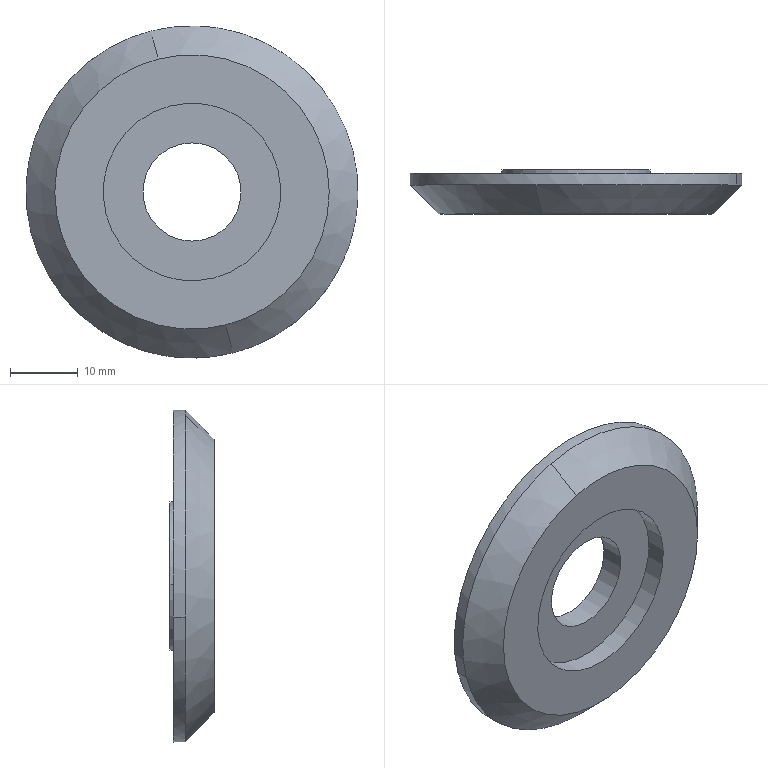Part | SolidWorks | features BaseBody 1 | 1 solid | 14 faces | box 49 x 6.5 x 49 mm | volume 7995 mm3 | cylinder 8 | plane 4 | cone 2 | commonest cylinder face diameters 14.5 x2 22 x2 26.2 x2 49 x2
STEP:
#1=CARTESIAN_POINT('',(-525.322,-118.5,-1.324));
#2=VERTEX_POINT('',#1);
#3=CARTESIAN_POINT('',(-535.321,-118.5,37.907));
#4=VERTEX_POINT('',#3);
#5=CARTESIAN_POINT('',(-530.322,-118.5,18.291));
#6=DIRECTION('',(0.,-1.,0.));
#7=DIRECTION('',(0.,0.,-1.));
#8=AXIS2_PLACEMENT_3D('',#5,#6,#7);
#9=CIRCLE('',#8,20.243);
#10=EDGE_CURVE('',#2,#4,#9,.T.);
#11=ORIENTED_EDGE('',*,*,#10,.F.);
#12=CARTESIAN_POINT('',(-524.27,-114.243,-5.45));
#13=VERTEX_POINT('',#12);
#14=CARTESIAN_POINT('',(-525.475,-119.121,-0.7223));
#15=DIRECTION('',(0.1747,0.7071,-0.6852));
#16=VECTOR('',#15,1000.);
#17=LINE('',#14,#16);
#18=EDGE_CURVE('',#2,#13,#17,.T.);
#19=ORIENTED_EDGE('',*,*,#18,.T.);
#20=CARTESIAN_POINT('',(-506.581,-114.243,24.343));
#21=VERTEX_POINT('',#20);
#22=CARTESIAN_POINT('',(-530.322,-114.243,18.291));
#23=DIRECTION('',(0.,1.,0.));
#24=DIRECTION('',(0.,0.,1.));
#25=AXIS2_PLACEMENT_3D('',#22,#23,#24);
#26=CIRCLE('',#25,24.5);
#27=EDGE_CURVE('',#21,#13,#26,.T.);
#28=ORIENTED_EDGE('',*,*,#27,.F.);
#29=CARTESIAN_POINT('',(-536.373,-114.243,42.032));
#30=VERTEX_POINT('',#29);
#31=CARTESIAN_POINT('',(-530.322,-114.243,18.291));
#32=DIRECTION('',(0.,1.,0.));
#33=DIRECTION('',(0.,0.,1.));
#34=AXIS2_PLACEMENT_3D('',#31,#32,#33);
#35=CIRCLE('',#34,24.5);
#36=EDGE_CURVE('',#30,#21,#35,.T.);
#37=ORIENTED_EDGE('',*,*,#36,.F.);
#38=CARTESIAN_POINT('',(-535.168,-119.121,37.304));
#39=DIRECTION('',(-0.1747,0.7071,0.6852));
#40=VECTOR('',#39,1000.);
#41=LINE('',#38,#40);
#42=EDGE_CURVE('',#4,#30,#41,.T.);
#43=ORIENTED_EDGE('',*,*,#42,.F.);
#44=EDGE_LOOP('',(#11,#19,#28,#37,#43));
#45=FACE_OUTER_BOUND('',#44,.T.);
#46=CARTESIAN_POINT('',(-530.322,-119.121,18.291));
#47=DIRECTION('',(0.,1.,0.));
#48=DIRECTION('',(-0.247,0.,0.969));
#49=AXIS2_PLACEMENT_3D('',#46,#47,#48);
#50=CONICAL_SURFACE('',#49,19.621,0.7854);
#51=ADVANCED_FACE('',(#45),#50,.T.);
#52=CARTESIAN_POINT('',(-537.528,-112.,17.495));
#53=VERTEX_POINT('',#52);
#54=CARTESIAN_POINT('',(-523.115,-112.,19.087));
#55=VERTEX_POINT('',#54);
#56=CARTESIAN_POINT('',(-530.322,-112.,18.291));
#57=DIRECTION('',(0.,1.,0.));
#58=DIRECTION('',(-0.994,0.,-0.1097));
#59=AXIS2_PLACEMENT_3D('',#56,#57,#58);
#60=CIRCLE('',#59,7.25);
#61=EDGE_CURVE('',#53,#55,#60,.T.);
#62=ORIENTED_EDGE('',*,*,#61,.T.);
#63=CARTESIAN_POINT('',(-523.115,-115.5,19.087));
#64=VERTEX_POINT('',#63);
#65=CARTESIAN_POINT('',(-523.115,-112.,19.087));
#66=DIRECTION('',(0.,-1.,0.));
#67=VECTOR('',#66,1000.);
#68=LINE('',#65,#67);
#69=EDGE_CURVE('',#55,#64,#68,.T.);
#70=ORIENTED_EDGE('',*,*,#69,.T.);
#71=CARTESIAN_POINT('',(-537.528,-115.5,17.495));
#72=VERTEX_POINT('',#71);
#73=CARTESIAN_POINT('',(-530.322,-115.5,18.291));
#74=DIRECTION('',(0.,-1.,0.));
#75=DIRECTION('',(0.969,0.,0.247));
#76=AXIS2_PLACEMENT_3D('',#73,#74,#75);
#77=CIRCLE('',#76,7.25);
#78=EDGE_CURVE('',#64,#72,#77,.T.);
#79=ORIENTED_EDGE('',*,*,#78,.T.);
#80=CARTESIAN_POINT('',(-537.528,-112.,17.495));
#81=DIRECTION('',(0.,-1.,0.));
#82=VECTOR('',#81,1000.);
#83=LINE('',#80,#82);
#84=EDGE_CURVE('',#53,#72,#83,.T.);
#85=ORIENTED_EDGE('',*,*,#84,.F.);
#86=EDGE_LOOP('',(#62,#70,#79,#85));
#87=FACE_OUTER_BOUND('',#86,.T.);
#88=CARTESIAN_POINT('',(-530.322,-112.,18.291));
#89=DIRECTION('',(0.,-1.,0.));
#90=DIRECTION('',(-0.994,0.,-0.1097));
#91=AXIS2_PLACEMENT_3D('',#88,#89,#90);
#92=CYLINDRICAL_SURFACE('',#91,7.25);
#93=ADVANCED_FACE('',(#87),#92,.F.);
#94=CARTESIAN_POINT('',(-541.255,-112.,17.084));
#95=VERTEX_POINT('',#94);
#96=CARTESIAN_POINT('',(-519.388,-112.,19.498));
#97=VERTEX_POINT('',#96);
#98=CARTESIAN_POINT('',(-530.322,-112.,18.291));
#99=DIRECTION('',(0.,-1.,0.));
#100=DIRECTION('',(-0.994,0.,-0.1097));
#101=AXIS2_PLACEMENT_3D('',#98,#99,#100);
#102=CIRCLE('',#101,11.);
#103=EDGE_CURVE('',#95,#97,#102,.T.);
#104=ORIENTED_EDGE('',*,*,#103,.T.);
#105=CARTESIAN_POINT('',(-519.388,-112.5,19.498));
#106=VERTEX_POINT('',#105);
#107=CARTESIAN_POINT('',(-519.388,-112.,19.498));
#108=DIRECTION('',(0.,-1.,0.));
#109=VECTOR('',#108,1000.);
#110=LINE('',#107,#109);
#111=EDGE_CURVE('',#97,#106,#110,.T.);
#112=ORIENTED_EDGE('',*,*,#111,.T.);
#113=CARTESIAN_POINT('',(-541.255,-112.5,17.084));
#114=VERTEX_POINT('',#113);
#115=CARTESIAN_POINT('',(-530.322,-112.5,18.291));
#116=DIRECTION('',(0.,-1.,0.));
#117=DIRECTION('',(-0.994,0.,-0.1097));
#118=AXIS2_PLACEMENT_3D('',#115,#116,#117);
#119=CIRCLE('',#118,11.);
#120=EDGE_CURVE('',#114,#106,#119,.T.);
#121=ORIENTED_EDGE('',*,*,#120,.F.);
#122=CARTESIAN_POINT('',(-541.255,-112.,17.084));
#123=DIRECTION('',(0.,-1.,0.));
#124=VECTOR('',#123,1000.);
#125=LINE('',#122,#124);
#126=EDGE_CURVE('',#95,#114,#125,.T.);
#127=ORIENTED_EDGE('',*,*,#126,.F.);
#128=EDGE_LOOP('',(#104,#112,#121,#127));
#129=FACE_OUTER_BOUND('',#128,.T.);
#130=CARTESIAN_POINT('',(-530.322,-112.,18.291));
#131=DIRECTION('',(0.,-1.,0.));
#132=DIRECTION('',(-0.994,0.,-0.1097));
#133=AXIS2_PLACEMENT_3D('',#130,#131,#132);
#134=CYLINDRICAL_SURFACE('',#133,11.);
#135=ADVANCED_FACE('',(#129),#134,.T.);
#136=CARTESIAN_POINT('',(-554.062,-112.5,12.24));
#137=VERTEX_POINT('',#136);
#138=CARTESIAN_POINT('',(-506.581,-112.5,24.343));
#139=VERTEX_POINT('',#138);
#140=CARTESIAN_POINT('',(-530.322,-112.5,18.291));
#141=DIRECTION('',(0.,-1.,0.));
#142=DIRECTION('',(0.,0.,-1.));
#143=AXIS2_PLACEMENT_3D('',#140,#141,#142);
#144=CIRCLE('',#143,24.5);
#145=EDGE_CURVE('',#137,#139,#144,.T.);
#146=ORIENTED_EDGE('',*,*,#145,.T.);
#147=CARTESIAN_POINT('',(-506.581,-112.5,24.343));
#148=DIRECTION('',(0.,-1.,0.));
#149=VECTOR('',#148,1000.);
#150=LINE('',#147,#149);
#151=EDGE_CURVE('',#139,#21,#150,.T.);
#152=ORIENTED_EDGE('',*,*,#151,.T.);
#153=ORIENTED_EDGE('',*,*,#27,.T.);
#154=CARTESIAN_POINT('',(-554.062,-114.243,12.24));
#155=VERTEX_POINT('',#154);
#156=CARTESIAN_POINT('',(-530.322,-114.243,18.291));
#157=DIRECTION('',(0.,1.,0.));
#158=DIRECTION('',(0.,0.,1.));
#159=AXIS2_PLACEMENT_3D('',#156,#157,#158);
#160=CIRCLE('',#159,24.5);
#161=EDGE_CURVE('',#13,#155,#160,.T.);
#162=ORIENTED_EDGE('',*,*,#161,.T.);
#163=CARTESIAN_POINT('',(-554.062,-112.5,12.24));
#164=DIRECTION('',(0.,-1.,0.));
#165=VECTOR('',#164,1000.);
#166=LINE('',#163,#165);
#167=EDGE_CURVE('',#137,#155,#166,.T.);
#168=ORIENTED_EDGE('',*,*,#167,.F.);
#169=EDGE_LOOP('',(#146,#152,#153,#162,#168));
#170=FACE_OUTER_BOUND('',#169,.T.);
#171=CARTESIAN_POINT('',(-530.322,-112.5,18.291));
#172=DIRECTION('',(0.,-1.,0.));
#173=DIRECTION('',(-0.969,0.,-0.247));
#174=AXIS2_PLACEMENT_3D('',#171,#172,#173);
#175=CYLINDRICAL_SURFACE('',#174,24.5);
#176=ADVANCED_FACE('',(#170),#175,.T.);
#177=CARTESIAN_POINT('',(-517.627,-115.5,21.527));
#178=VERTEX_POINT('',#177);
#179=CARTESIAN_POINT('',(-543.016,-115.5,15.055));
#180=VERTEX_POINT('',#179);
#181=CARTESIAN_POINT('',(-530.322,-115.5,18.291));
#182=DIRECTION('',(0.,-1.,0.));
#183=DIRECTION('',(0.,0.,-1.));
#184=AXIS2_PLACEMENT_3D('',#181,#182,#183);
#185=CIRCLE('',#184,13.1);
#186=EDGE_CURVE('',#178,#180,#185,.T.);
#187=ORIENTED_EDGE('',*,*,#186,.F.);
#188=CARTESIAN_POINT('',(-517.627,-118.5,21.527));
#189=VERTEX_POINT('',#188);
#190=CARTESIAN_POINT('',(-517.627,-118.5,21.527));
#191=DIRECTION('',(0.,-1.,0.));
#192=VECTOR('',#191,1000.);
#193=LINE('',#190,#192);
#194=EDGE_CURVE('',#178,#189,#193,.T.);
#195=ORIENTED_EDGE('',*,*,#194,.T.);
#196=CARTESIAN_POINT('',(-543.016,-118.5,15.055));
#197=VERTEX_POINT('',#196);
#198=CARTESIAN_POINT('',(-530.322,-118.5,18.291));
#199=DIRECTION('',(0.,-1.,0.));
#200=DIRECTION('',(0.,0.,-1.));
#201=AXIS2_PLACEMENT_3D('',#198,#199,#200);
#202=CIRCLE('',#201,13.1);
#203=EDGE_CURVE('',#189,#197,#202,.T.);
#204=ORIENTED_EDGE('',*,*,#203,.T.);
#205=CARTESIAN_POINT('',(-543.016,-118.5,15.055));
#206=DIRECTION('',(0.,-1.,0.));
#207=VECTOR('',#206,1000.);
#208=LINE('',#205,#207);
#209=EDGE_CURVE('',#180,#197,#208,.T.);
#210=ORIENTED_EDGE('',*,*,#209,.F.);
#211=EDGE_LOOP('',(#187,#195,#204,#210));
#212=FACE_OUTER_BOUND('',#211,.T.);
#213=CARTESIAN_POINT('',(-530.322,-118.5,18.291));
#214=DIRECTION('',(0.,-1.,0.));
#215=DIRECTION('',(-0.969,0.,-0.247));
#216=AXIS2_PLACEMENT_3D('',#213,#214,#215);
#217=CYLINDRICAL_SURFACE('',#216,13.1);
#218=ADVANCED_FACE('',(#212),#217,.F.);
#219=ORIENTED_EDGE('',*,*,#61,.F.);
#220=CARTESIAN_POINT('',(-530.322,-112.,18.291));
#221=DIRECTION('',(0.,1.,0.));
#222=DIRECTION('',(-0.994,0.,-0.1097));
#223=AXIS2_PLACEMENT_3D('',#220,#221,#222);
#224=CIRCLE('',#223,7.25);
#225=EDGE_CURVE('',#55,#53,#224,.T.);
#226=ORIENTED_EDGE('',*,*,#225,.F.);
#227=EDGE_LOOP('',(#219,#226));
#228=FACE_BOUND('',#227,.T.);
#229=ORIENTED_EDGE('',*,*,#103,.F.);
#230=CARTESIAN_POINT('',(-530.322,-112.,18.291));
#231=DIRECTION('',(0.,-1.,0.));
#232=DIRECTION('',(-0.994,0.,-0.1097));
#233=AXIS2_PLACEMENT_3D('',#230,#231,#232);
#234=CIRCLE('',#233,11.);
#235=EDGE_CURVE('',#97,#95,#234,.T.);
#236=ORIENTED_EDGE('',*,*,#235,.F.);
#237=EDGE_LOOP('',(#229,#236));
#238=FACE_OUTER_BOUND('',#237,.T.);
#239=CARTESIAN_POINT('',(-530.322,-112.,18.291));
#240=DIRECTION('',(0.,-1.,0.));
#241=DIRECTION('',(0.,0.,-1.));
#242=AXIS2_PLACEMENT_3D('',#239,#240,#241);
#243=PLANE('',#242);
#244=ADVANCED_FACE('',(#228,#238),#243,.F.);
#245=CARTESIAN_POINT('',(-530.322,-115.5,18.291));
#246=DIRECTION('',(0.,-1.,0.));
#247=DIRECTION('',(0.969,0.,0.247));
#248=AXIS2_PLACEMENT_3D('',#245,#246,#247);
#249=CIRCLE('',#248,7.25);
#250=EDGE_CURVE('',#72,#64,#249,.T.);
#251=ORIENTED_EDGE('',*,*,#250,.F.);
#252=ORIENTED_EDGE('',*,*,#78,.F.);
#253=EDGE_LOOP('',(#251,#252));
#254=FACE_BOUND('',#253,.T.);
#255=CARTESIAN_POINT('',(-530.322,-115.5,18.291));
#256=DIRECTION('',(0.,-1.,0.));
#257=DIRECTION('',(0.,0.,-1.));
#258=AXIS2_PLACEMENT_3D('',#255,#256,#257);
#259=CIRCLE('',#258,13.1);
#260=EDGE_CURVE('',#180,#178,#259,.T.);
#261=ORIENTED_EDGE('',*,*,#260,.T.);
#262=ORIENTED_EDGE('',*,*,#186,.T.);
#263=EDGE_LOOP('',(#261,#262));
#264=FACE_OUTER_BOUND('',#263,.T.);
#265=CARTESIAN_POINT('',(-12.902,-115.5,135.432));
#266=DIRECTION('',(0.,-1.,0.));
#267=DIRECTION('',(0.,0.,-1.));
#268=AXIS2_PLACEMENT_3D('',#265,#266,#267);
#269=PLANE('',#268);
#270=ADVANCED_FACE('',(#254,#264),#269,.T.);
#271=ORIENTED_EDGE('',*,*,#194,.F.);
#272=ORIENTED_EDGE('',*,*,#260,.F.);
#273=ORIENTED_EDGE('',*,*,#209,.T.);
#274=CARTESIAN_POINT('',(-530.322,-118.5,18.291));
#275=DIRECTION('',(0.,-1.,0.));
#276=DIRECTION('',(0.,0.,-1.));
#277=AXIS2_PLACEMENT_3D('',#274,#275,#276);
#278=CIRCLE('',#277,13.1);
#279=EDGE_CURVE('',#197,#189,#278,.T.);
#280=ORIENTED_EDGE('',*,*,#279,.T.);
#281=EDGE_LOOP('',(#271,#272,#273,#280));
#282=FACE_OUTER_BOUND('',#281,.T.);
#283=CARTESIAN_POINT('',(-530.322,-118.5,18.291));
#284=DIRECTION('',(0.,-1.,0.));
#285=DIRECTION('',(-0.969,0.,-0.247));
#286=AXIS2_PLACEMENT_3D('',#283,#284,#285);
#287=CYLINDRICAL_SURFACE('',#286,13.1);
#288=ADVANCED_FACE('',(#282),#287,.F.);
#289=ORIENTED_EDGE('',*,*,#279,.F.);
#290=ORIENTED_EDGE('',*,*,#203,.F.);
#291=EDGE_LOOP('',(#289,#290));
#292=FACE_BOUND('',#291,.T.);
#293=CARTESIAN_POINT('',(-530.322,-118.5,18.291));
#294=DIRECTION('',(0.,-1.,0.));
#295=DIRECTION('',(0.,0.,-1.));
#296=AXIS2_PLACEMENT_3D('',#293,#294,#295);
#297=CIRCLE('',#296,20.243);
#298=EDGE_CURVE('',#4,#2,#297,.T.);
#299=ORIENTED_EDGE('',*,*,#298,.T.);
#300=ORIENTED_EDGE('',*,*,#10,.T.);
#301=EDGE_LOOP('',(#299,#300));
#302=FACE_OUTER_BOUND('',#301,.T.);
#303=CARTESIAN_POINT('',(-12.902,-118.5,135.432));
#304=DIRECTION('',(0.,-1.,0.));
#305=DIRECTION('',(0.,0.,-1.));
#306=AXIS2_PLACEMENT_3D('',#303,#304,#305);
#307=PLANE('',#306);
#308=ADVANCED_FACE('',(#292,#302),#307,.T.);
#309=ORIENTED_EDGE('',*,*,#151,.F.);
#310=CARTESIAN_POINT('',(-530.322,-112.5,18.291));
#311=DIRECTION('',(0.,-1.,0.));
#312=DIRECTION('',(0.,0.,-1.));
#313=AXIS2_PLACEMENT_3D('',#310,#311,#312);
#314=CIRCLE('',#313,24.5);
#315=EDGE_CURVE('',#139,#137,#314,.T.);
#316=ORIENTED_EDGE('',*,*,#315,.T.);
#317=ORIENTED_EDGE('',*,*,#167,.T.);
#318=CARTESIAN_POINT('',(-530.322,-114.243,18.291));
#319=DIRECTION('',(0.,1.,0.));
#320=DIRECTION('',(0.,0.,1.));
#321=AXIS2_PLACEMENT_3D('',#318,#319,#320);
#322=CIRCLE('',#321,24.5);
#323=EDGE_CURVE('',#155,#30,#322,.T.);
#324=ORIENTED_EDGE('',*,*,#323,.T.);
#325=ORIENTED_EDGE('',*,*,#36,.T.);
#326=EDGE_LOOP('',(#309,#316,#317,#324,#325));
#327=FACE_OUTER_BOUND('',#326,.T.);
#328=CARTESIAN_POINT('',(-530.322,-112.5,18.291));
#329=DIRECTION('',(0.,-1.,0.));
#330=DIRECTION('',(-0.969,0.,-0.247));
#331=AXIS2_PLACEMENT_3D('',#328,#329,#330);
#332=CYLINDRICAL_SURFACE('',#331,24.5);
#333=ADVANCED_FACE('',(#327),#332,.T.);
#334=ORIENTED_EDGE('',*,*,#120,.T.);
#335=CARTESIAN_POINT('',(-530.322,-112.5,18.291));
#336=DIRECTION('',(0.,-1.,0.));
#337=DIRECTION('',(-0.994,0.,-0.1097));
#338=AXIS2_PLACEMENT_3D('',#335,#336,#337);
#339=CIRCLE('',#338,11.);
#340=EDGE_CURVE('',#106,#114,#339,.T.);
#341=ORIENTED_EDGE('',*,*,#340,.T.);
#342=EDGE_LOOP('',(#334,#341));
#343=FACE_BOUND('',#342,.T.);
#344=ORIENTED_EDGE('',*,*,#145,.F.);
#345=ORIENTED_EDGE('',*,*,#315,.F.);
#346=EDGE_LOOP('',(#344,#345));
#347=FACE_OUTER_BOUND('',#346,.T.);
#348=CARTESIAN_POINT('',(-12.902,-112.5,135.432));
#349=DIRECTION('',(0.,-1.,0.));
#350=DIRECTION('',(0.,0.,-1.));
#351=AXIS2_PLACEMENT_3D('',#348,#349,#350);
#352=PLANE('',#351);
#353=ADVANCED_FACE('',(#343,#347),#352,.F.);
#354=ORIENTED_EDGE('',*,*,#111,.F.);
#355=ORIENTED_EDGE('',*,*,#235,.T.);
#356=ORIENTED_EDGE('',*,*,#126,.T.);
#357=ORIENTED_EDGE('',*,*,#340,.F.);
#358=EDGE_LOOP('',(#354,#355,#356,#357));
#359=FACE_OUTER_BOUND('',#358,.T.);
#360=CARTESIAN_POINT('',(-530.322,-112.,18.291));
#361=DIRECTION('',(0.,-1.,0.));
#362=DIRECTION('',(-0.994,0.,-0.1097));
#363=AXIS2_PLACEMENT_3D('',#360,#361,#362);
#364=CYLINDRICAL_SURFACE('',#363,11.);
#365=ADVANCED_FACE('',(#359),#364,.T.);
#366=ORIENTED_EDGE('',*,*,#69,.F.);
#367=ORIENTED_EDGE('',*,*,#225,.T.);
#368=ORIENTED_EDGE('',*,*,#84,.T.);
#369=ORIENTED_EDGE('',*,*,#250,.T.);
#370=EDGE_LOOP('',(#366,#367,#368,#369));
#371=FACE_OUTER_BOUND('',#370,.T.);
#372=CARTESIAN_POINT('',(-530.322,-112.,18.291));
#373=DIRECTION('',(0.,-1.,0.));
#374=DIRECTION('',(-0.994,0.,-0.1097));
#375=AXIS2_PLACEMENT_3D('',#372,#373,#374);
#376=CYLINDRICAL_SURFACE('',#375,7.25);
#377=ADVANCED_FACE('',(#371),#376,.F.);
#378=ORIENTED_EDGE('',*,*,#18,.F.);
#379=ORIENTED_EDGE('',*,*,#298,.F.);
#380=ORIENTED_EDGE('',*,*,#42,.T.);
#381=ORIENTED_EDGE('',*,*,#323,.F.);
#382=ORIENTED_EDGE('',*,*,#161,.F.);
#383=EDGE_LOOP('',(#378,#379,#380,#381,#382));
#384=FACE_OUTER_BOUND('',#383,.T.);
#385=CARTESIAN_POINT('',(-530.322,-119.121,18.291));
#386=DIRECTION('',(0.,1.,0.));
#387=DIRECTION('',(-0.247,0.,0.969));
#388=AXIS2_PLACEMENT_3D('',#385,#386,#387);
#389=CONICAL_SURFACE('',#388,19.621,0.7854);
#390=ADVANCED_FACE('',(#384),#389,.T.);
#391=CLOSED_SHELL('',(#51,#93,#135,#176,#218,#244,#270,#288,#308,#333,#353,#365,#377,#390));
#392=MANIFOLD_SOLID_BREP('',#391);
#393=CARTESIAN_POINT('',(0.,0.,0.));
#394=DIRECTION('',(0.,0.,1.));
#395=DIRECTION('',(1.,0.,0.));
#396=AXIS2_PLACEMENT_3D('',#393,#394,#395);
#397=(LENGTH_UNIT()NAMED_UNIT(*)SI_UNIT(.MILLI.,.METRE.));
#398=UNCERTAINTY_MEASURE_WITH_UNIT(LENGTH_MEASURE(0.00001),#397,'','');
#399=(NAMED_UNIT(*)PLANE_ANGLE_UNIT()SI_UNIT($,.RADIAN.));
#400=(NAMED_UNIT(*)SI_UNIT($,.STERADIAN.)SOLID_ANGLE_UNIT());
#401=(GEOMETRIC_REPRESENTATION_CONTEXT(3)GLOBAL_UNCERTAINTY_ASSIGNED_CONTEXT((#398))GLOBAL_UNIT_ASSIGNED_CONTEXT((#397,#399,#400))REPRESENTATION_CONTEXT('',''));
#402=ADVANCED_BREP_SHAPE_REPRESENTATION('',(#392,#396),#401);